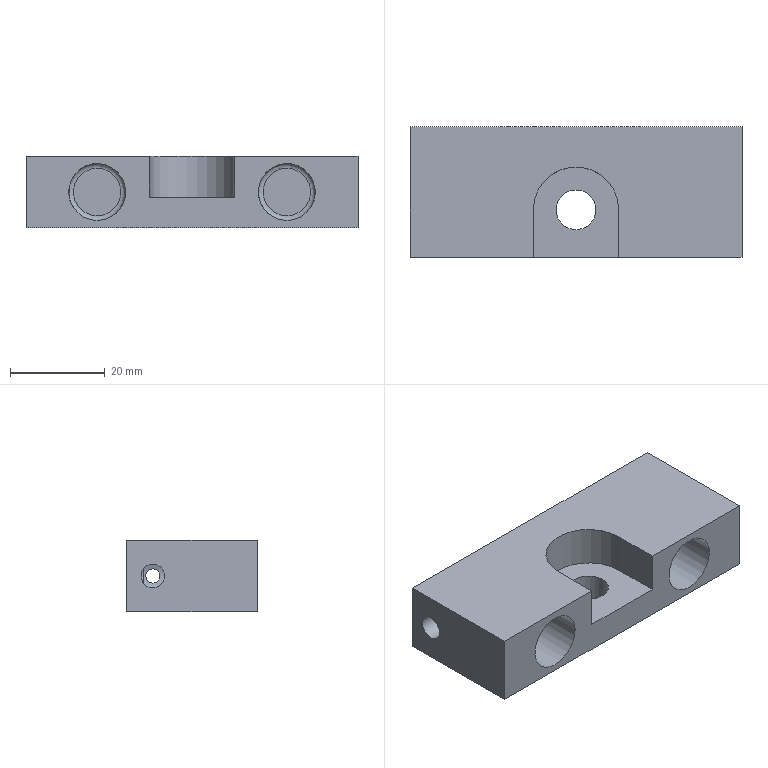NC program | NX | posted with a generic post | part box 70 x 27.5 x 15 mm
Whole program:
N10 G17 G21 G94 G90
(DRILLING_3 , TOOL : 点孔D10-150-90度)
N12 T07 M6
N14 G54
N16 G17 G0 G90 X22. Y7.5 B0. C0. S1600 M3
N18 G43 Z20. H7
N20 G94 G81 G99 Z-1.5 B-180. C90. F150. R3.
N22 G80
N24 G0 X22. Y7.5 Z20.
N26 M5
(DRILLING_2_COPY , TOOL : 钻头D5.1-62-92)
N28 T08 M6
N30 G54
N32 G17 G0 G90 X22. Y7.5 B0. C0. S1800 M3
N34 G43 Z20. H8
N36 G94 G83 G99 Z-20. B-180. C90. F150. Q2. R3.
N38 G80
N40 G0 X22. Y7.5 Z20.
N42 M5
(DRILLING_2_COPY_COPY , TOOL : 上排M6-23-D6-63)
N44 T10 M6
N46 G54
N48 G17 G0 G90 X22. Y7.5 B0. C0. S300 M3
N50 G43 Z20. H10
N52 G84 G94 G99 Z-5. B-180. C90. F300. R3.
N54 G80
N56 G0 X22. Y7.5 Z20.
N58 M5
N60 M2